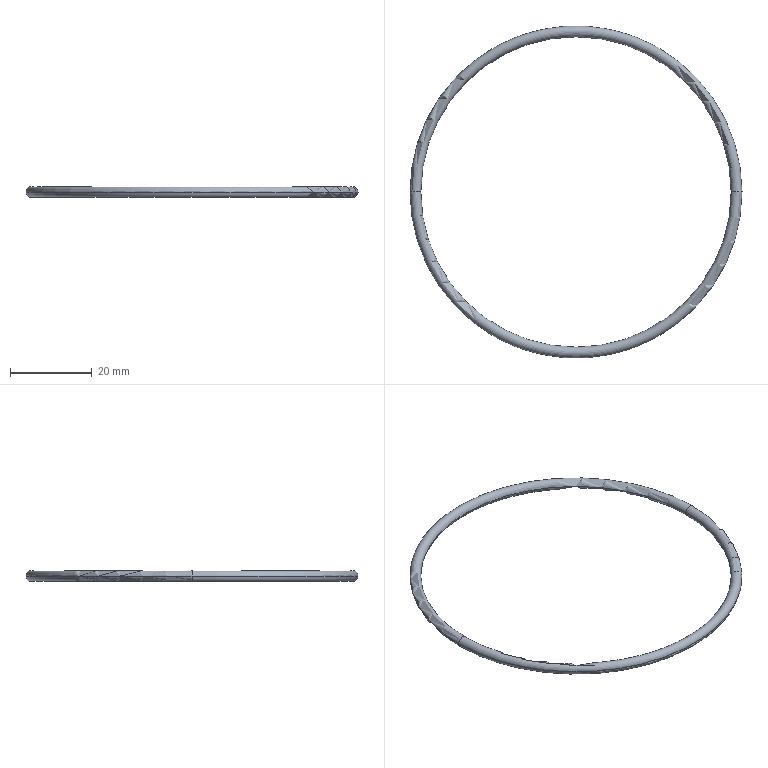Part | STEP file | MIFENGQUAN_14_1_1_1 | 1 solid | 4 faces | box 81.15 x 81.15 x 2.65 mm | volume 1360 mm3 | torus 4
STEP:
#1=CARTESIAN_POINT('',(0.,0.,0.));
#2=DIRECTION('',(0.,0.,1.));
#3=DIRECTION('',(1.,0.,0.));
#4=AXIS2_PLACEMENT_3D('',#1,#2,#3);
#5=CARTESIAN_POINT('',(-37.925,0.,0.));
#6=VERTEX_POINT('',#5);
#7=CARTESIAN_POINT('',(-40.575,0.,0.));
#8=VERTEX_POINT('',#7);
#9=CARTESIAN_POINT('',(-39.25,0.,0.));
#10=DIRECTION('',(0.,1.,0.));
#11=DIRECTION('',(1.,0.,0.));
#12=AXIS2_PLACEMENT_3D('',#9,#10,#11);
#13=CIRCLE('',#12,1.325);
#14=EDGE_CURVE('',#6,#8,#13,.T.);
#15=ORIENTED_EDGE('',*,*,#14,.T.);
#16=CARTESIAN_POINT('',(40.575,0.,0.));
#17=VERTEX_POINT('',#16);
#18=CARTESIAN_POINT('',(0.,0.,0.));
#19=DIRECTION('',(0.,0.,1.));
#20=DIRECTION('',(-1.,0.,0.));
#21=AXIS2_PLACEMENT_3D('',#18,#19,#20);
#22=CIRCLE('',#21,40.575);
#23=EDGE_CURVE('',#8,#17,#22,.T.);
#24=ORIENTED_EDGE('',*,*,#23,.T.);
#25=CARTESIAN_POINT('',(37.925,0.,0.));
#26=VERTEX_POINT('',#25);
#27=CARTESIAN_POINT('',(39.25,0.,0.));
#28=DIRECTION('',(0.,-1.,0.));
#29=DIRECTION('',(-1.,0.,0.));
#30=AXIS2_PLACEMENT_3D('',#27,#28,#29);
#31=CIRCLE('',#30,1.325);
#32=EDGE_CURVE('',#26,#17,#31,.T.);
#33=ORIENTED_EDGE('',*,*,#32,.F.);
#34=CARTESIAN_POINT('',(0.,0.,0.));
#35=DIRECTION('',(0.,0.,1.));
#36=DIRECTION('',(-1.,0.,0.));
#37=AXIS2_PLACEMENT_3D('',#34,#35,#36);
#38=CIRCLE('',#37,37.925);
#39=EDGE_CURVE('',#6,#26,#38,.T.);
#40=ORIENTED_EDGE('',*,*,#39,.F.);
#41=EDGE_LOOP('',(#15,#24,#33,#40));
#42=FACE_OUTER_BOUND('',#41,.F.);
#43=CARTESIAN_POINT('',(0.,0.,0.));
#44=DIRECTION('',(0.,0.,1.));
#45=DIRECTION('',(-1.,0.,0.));
#46=AXIS2_PLACEMENT_3D('',#43,#44,#45);
#47=TOROIDAL_SURFACE('',#46,39.25,1.325);
#48=ADVANCED_FACE('',(#42),#47,.T.);
#49=ORIENTED_EDGE('',*,*,#14,.F.);
#50=CARTESIAN_POINT('',(0.,0.,0.));
#51=DIRECTION('',(0.,0.,-1.));
#52=DIRECTION('',(-1.,0.,0.));
#53=AXIS2_PLACEMENT_3D('',#50,#51,#52);
#54=CIRCLE('',#53,37.925);
#55=EDGE_CURVE('',#6,#26,#54,.T.);
#56=ORIENTED_EDGE('',*,*,#55,.T.);
#57=ORIENTED_EDGE('',*,*,#32,.T.);
#58=CARTESIAN_POINT('',(0.,0.,0.));
#59=DIRECTION('',(0.,0.,-1.));
#60=DIRECTION('',(-1.,0.,0.));
#61=AXIS2_PLACEMENT_3D('',#58,#59,#60);
#62=CIRCLE('',#61,40.575);
#63=EDGE_CURVE('',#8,#17,#62,.T.);
#64=ORIENTED_EDGE('',*,*,#63,.F.);
#65=EDGE_LOOP('',(#49,#56,#57,#64));
#66=FACE_OUTER_BOUND('',#65,.F.);
#67=CARTESIAN_POINT('',(0.,0.,0.));
#68=DIRECTION('',(0.,0.,1.));
#69=DIRECTION('',(-1.,0.,0.));
#70=AXIS2_PLACEMENT_3D('',#67,#68,#69);
#71=TOROIDAL_SURFACE('',#70,39.25,1.325);
#72=ADVANCED_FACE('',(#66),#71,.T.);
#73=CARTESIAN_POINT('',(-39.25,0.,0.));
#74=DIRECTION('',(0.,1.,0.));
#75=DIRECTION('',(-1.,0.,0.));
#76=AXIS2_PLACEMENT_3D('',#73,#74,#75);
#77=CIRCLE('',#76,1.325);
#78=EDGE_CURVE('',#8,#6,#77,.T.);
#79=ORIENTED_EDGE('',*,*,#78,.F.);
#80=ORIENTED_EDGE('',*,*,#63,.T.);
#81=CARTESIAN_POINT('',(39.25,0.,0.));
#82=DIRECTION('',(0.,-1.,0.));
#83=DIRECTION('',(1.,0.,0.));
#84=AXIS2_PLACEMENT_3D('',#81,#82,#83);
#85=CIRCLE('',#84,1.325);
#86=EDGE_CURVE('',#17,#26,#85,.T.);
#87=ORIENTED_EDGE('',*,*,#86,.T.);
#88=ORIENTED_EDGE('',*,*,#55,.F.);
#89=EDGE_LOOP('',(#79,#80,#87,#88));
#90=FACE_OUTER_BOUND('',#89,.F.);
#91=CARTESIAN_POINT('',(0.,0.,0.));
#92=DIRECTION('',(0.,0.,1.));
#93=DIRECTION('',(-1.,0.,0.));
#94=AXIS2_PLACEMENT_3D('',#91,#92,#93);
#95=TOROIDAL_SURFACE('',#94,39.25,1.325);
#96=ADVANCED_FACE('',(#90),#95,.T.);
#97=ORIENTED_EDGE('',*,*,#78,.T.);
#98=ORIENTED_EDGE('',*,*,#39,.T.);
#99=ORIENTED_EDGE('',*,*,#86,.F.);
#100=ORIENTED_EDGE('',*,*,#23,.F.);
#101=EDGE_LOOP('',(#97,#98,#99,#100));
#102=FACE_OUTER_BOUND('',#101,.F.);
#103=CARTESIAN_POINT('',(0.,0.,0.));
#104=DIRECTION('',(0.,0.,1.));
#105=DIRECTION('',(-1.,0.,0.));
#106=AXIS2_PLACEMENT_3D('',#103,#104,#105);
#107=TOROIDAL_SURFACE('',#106,39.25,1.325);
#108=ADVANCED_FACE('',(#102),#107,.T.);
#109=CLOSED_SHELL('',(#48,#72,#96,#108));
#110=MANIFOLD_SOLID_BREP('',#109);
#111=(LENGTH_UNIT()NAMED_UNIT(*)SI_UNIT(.MILLI.,.METRE.));
#112=UNCERTAINTY_MEASURE_WITH_UNIT(LENGTH_MEASURE(0.01148),#111,'','');
#113=(NAMED_UNIT(*)PLANE_ANGLE_UNIT()SI_UNIT($,.RADIAN.));
#114=PLANE_ANGLE_MEASURE_WITH_UNIT(PLANE_ANGLE_MEASURE(0.01745),#113);
#115=(CONVERSION_BASED_UNIT('DEGREE',#114)NAMED_UNIT(*)PLANE_ANGLE_UNIT());
#116=(NAMED_UNIT(*)SI_UNIT($,.STERADIAN.)SOLID_ANGLE_UNIT());
#117=(GEOMETRIC_REPRESENTATION_CONTEXT(3)GLOBAL_UNCERTAINTY_ASSIGNED_CONTEXT((#112))GLOBAL_UNIT_ASSIGNED_CONTEXT((#111,#115,#116))REPRESENTATION_CONTEXT('',''));
#118=ADVANCED_BREP_SHAPE_REPRESENTATION('',(#4,#110),#117);